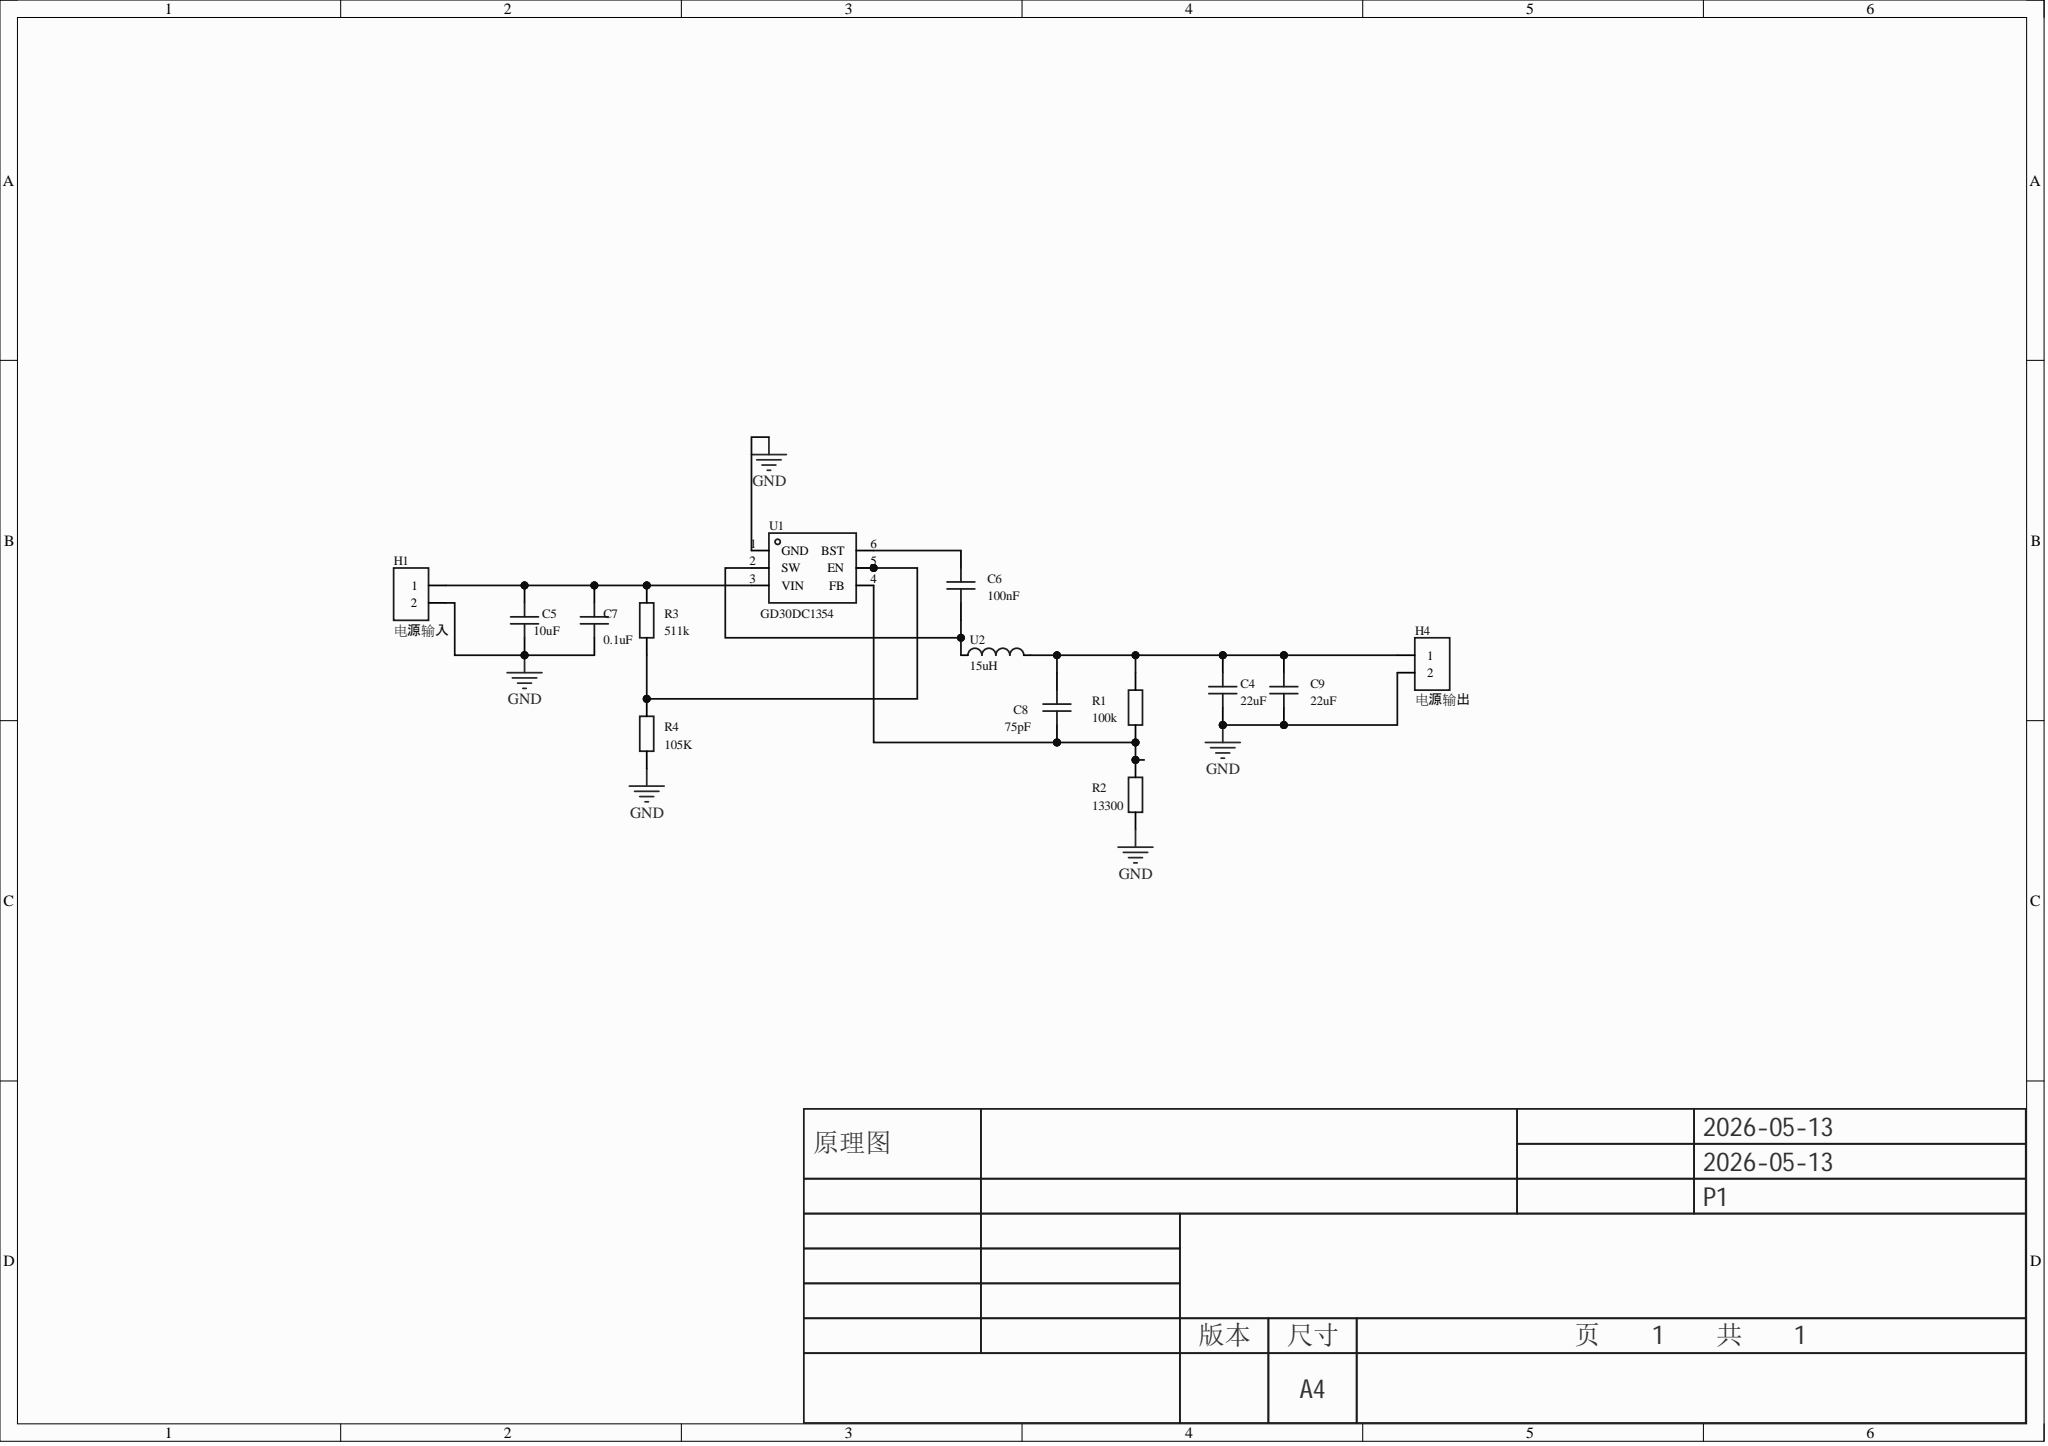Circuit board | Altium Designer | 14 parts | 7 nets
Bill of materials:
Comment,Description,Designator,Footprint,LibRef,Quantity
"22uF","","C4, C9","C0805","CAP_0805","2"
"10uF","","C5","C0805","CAP_0805","1"
"100nF","","C6","C0805","CAP_0805","1"
"0.1uF","","C7","C0805","CAP_0805","1"
"75pF","","C8","C0805","CAP_0805","1"
"电源输入","","H1","HDR-TH_2P-P2.54-V-F","HDR-F_2.54_1x2P","1"
"电源输出","","H4","HDR-TH_2P-P2.54-V-F","HDR-F_2.54_1x2P","1"
"100k","","R1","R0805","Res_0805","1"
"13300","","R2","R0805","Res_0805","1"
"511k","","R3","R0805","Res_0805","1"
"105K","","R4","R0805","Res_0805","1"
"GD30DC1354","","U1","SOT-23-6_L2.9-W1.7-P0.95-LS2.8-BL","GD30DC1354","1"
"15uH","","U2","IND-SMD_L6.6-W6.6","15uH","1"
Netlist (Protel format):
[
C4
C0805
22uF



]
[
C5
C0805
10uF



]
[
C6
C0805
100nF



]
[
C7
C0805
0.1uF



]
[
C8
C0805
75pF



]
[
C9
C0805
22uF



]
[
H1
HDR-TH_2P-P2.54-V-F
电源输入



]
[
H4
HDR-TH_2P-P2.54-V-F
电源输出



]
[
R1
R0805
100k



]
[
R2
R0805
13300



]
[
R3
R0805
511k



]
[
R4
R0805
105K



]
[
U1
SOT-23-6_L2.9-W1.7-P0.95-LS2.8-BL
GD30DC1354



]
[
U2
IND-SMD_L6.6-W6.6
15uH



]
(
NetR3_2
R3-2
R4-2
U1-5
)
(
NetC8_1
C8-1
R1-1
R2-2
U1-4
)
(
NetC6_2
C6-2
U1-6
)
(
NetC6_1
C6-1
U1-2
U2-1
)
(
NetC5_1
C5-1
C7-2
H1-1
R3-1
U1-3
)
(
NetC4_2
C4-2
C8-2
C9-2
H4-1
R1-2
U2-2
)
(
GND
C4-1
C5-2
C7-1
C9-1
H1-2
H4-2
R2-1
R4-1
U1-1
)